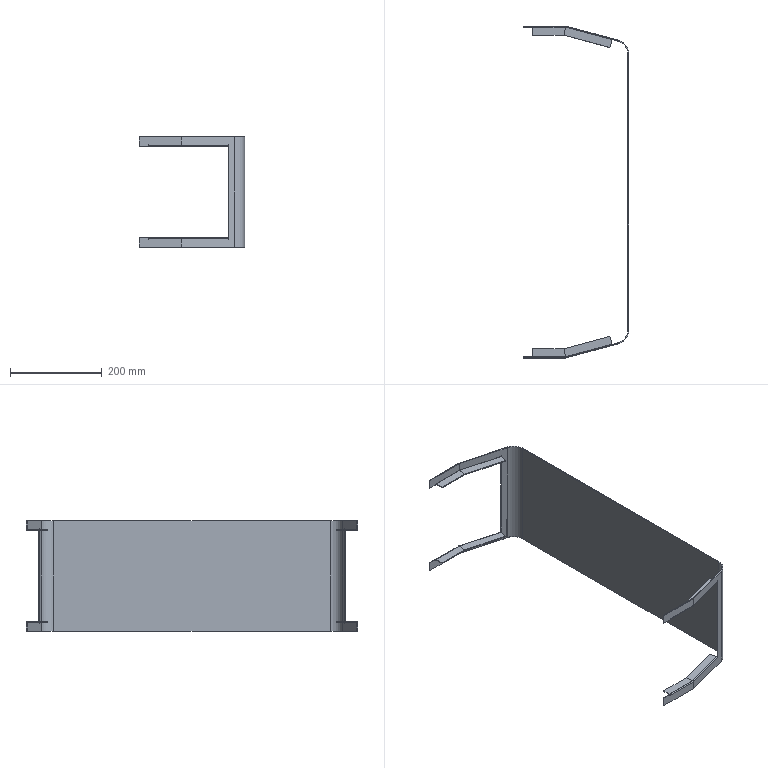Part | SolidWorks | features EdgeFlange 2, MirrorPattern 2, FlatPattern 1, ICE 1, SMBaseFlange 1, SheetMetal 1 | 1 solid | 166 faces | box 229.9 x 723 x 240 mm | volume 395484 mm3 | plane 130 | cylinder 28 | spline 8 | commonest cylinder face diameters 0.4 x12 4.4 x12 55.8 x2 59.8 x2